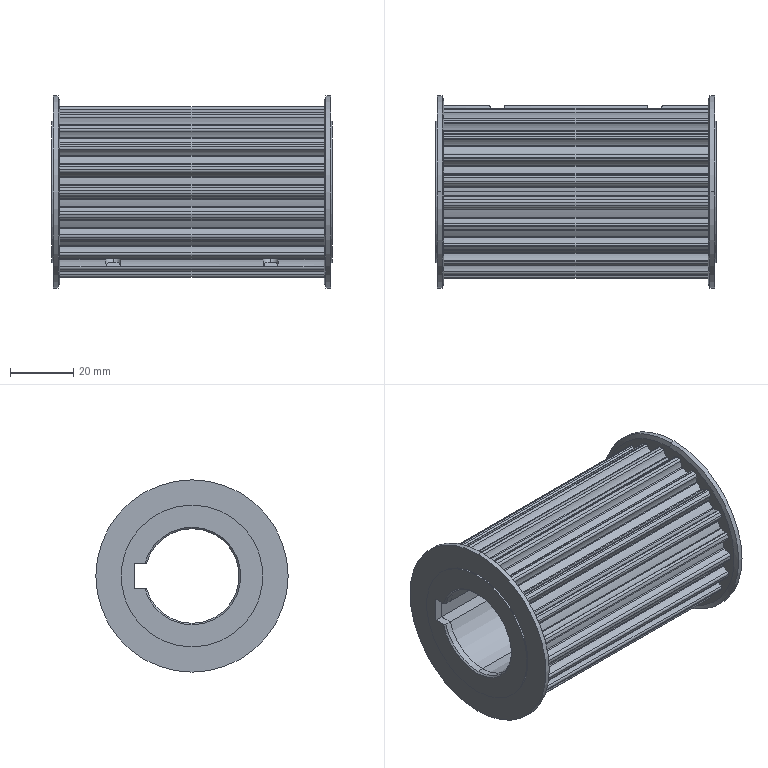Part | SolidWorks | 3 solids | 281 faces | box 89 x 61 x 61 mm | volume 120828 mm3 | cylinder 252 | plane 19 | cone 10 | commonest cylinder face diameters 0.8 x60 1.5 x60 10.6 x54 48.99 x29 54.65 x24 30 x9